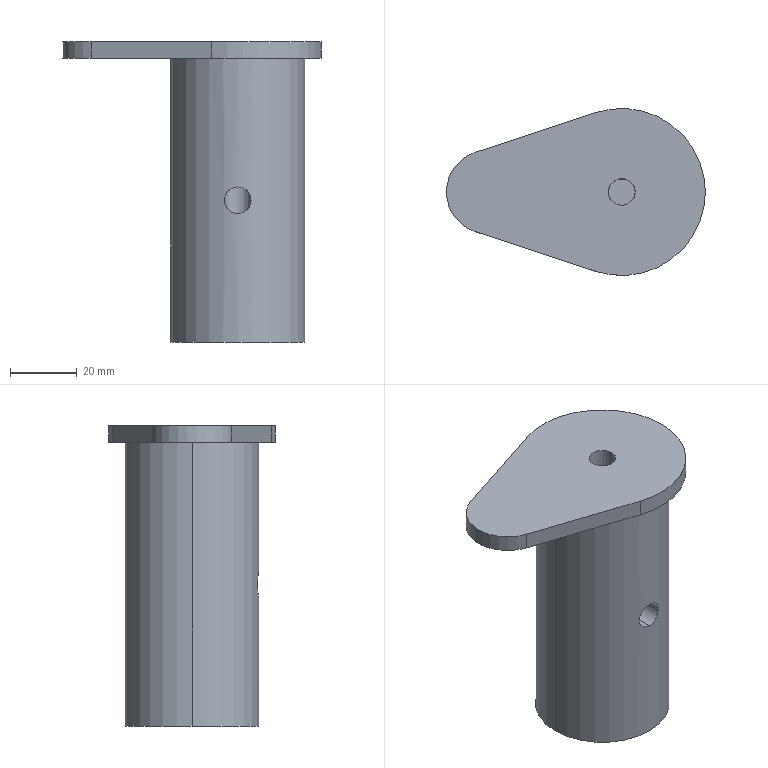Part | SolidWorks | features ICE 3, Extrusion 1 | 1 solid | 16 faces | box 77.5 x 50 x 90 mm | volume 116974 mm3 | cylinder 10 | plane 6 | commonest cylinder face diameters 8 x5 40 x2 50 x2 25 x1
STEP:
#1=CARTESIAN_POINT('',(0.,-20.,38.5));
#2=VERTEX_POINT('',#1);
#3=CARTESIAN_POINT('',(0.,-20.,46.5));
#4=VERTEX_POINT('',#3);
#5=CARTESIAN_POINT('',(0.,-20.,38.5));
#6=CARTESIAN_POINT('',(-0.2614,-20.,38.5));
#7=CARTESIAN_POINT('',(-0.5216,-19.995,38.525));
#8=CARTESIAN_POINT('',(-1.04,-19.975,38.628));
#9=CARTESIAN_POINT('',(-1.291,-19.96,38.705));
#10=CARTESIAN_POINT('',(-1.773,-19.923,38.905));
#11=CARTESIAN_POINT('',(-2.006,-19.9,39.03));
#12=CARTESIAN_POINT('',(-2.441,-19.852,39.321));
#13=CARTESIAN_POINT('',(-2.642,-19.826,39.486));
#14=CARTESIAN_POINT('',(-3.011,-19.773,39.854));
#15=CARTESIAN_POINT('',(-3.18,-19.746,40.059));
#16=CARTESIAN_POINT('',(-3.469,-19.697,40.492));
#17=CARTESIAN_POINT('',(-3.593,-19.675,40.722));
#18=CARTESIAN_POINT('',(-3.794,-19.637,41.207));
#19=CARTESIAN_POINT('',(-3.871,-19.622,41.46));
#20=CARTESIAN_POINT('',(-3.974,-19.601,41.972));
#21=CARTESIAN_POINT('',(-4.,-19.596,42.234));
#22=CARTESIAN_POINT('',(-4.,-19.596,42.762));
#23=CARTESIAN_POINT('',(-3.974,-19.601,43.022));
#24=CARTESIAN_POINT('',(-3.873,-19.622,43.535));
#25=CARTESIAN_POINT('',(-3.795,-19.637,43.79));
#26=CARTESIAN_POINT('',(-3.595,-19.674,44.273));
#27=CARTESIAN_POINT('',(-3.472,-19.697,44.503));
#28=CARTESIAN_POINT('',(-3.182,-19.746,44.938));
#29=CARTESIAN_POINT('',(-3.014,-19.772,45.143));
#30=CARTESIAN_POINT('',(-2.647,-19.825,45.511));
#31=CARTESIAN_POINT('',(-2.445,-19.851,45.676));
#32=CARTESIAN_POINT('',(-2.007,-19.9,45.97));
#33=CARTESIAN_POINT('',(-1.777,-19.922,46.093));
#34=CARTESIAN_POINT('',(-1.296,-19.959,46.293));
#35=CARTESIAN_POINT('',(-1.043,-19.974,46.371));
#36=CARTESIAN_POINT('',(-0.5264,-19.995,46.474));
#37=CARTESIAN_POINT('',(-0.2649,-20.,46.5));
#38=CARTESIAN_POINT('',(0.,-20.,46.5));
#39=B_SPLINE_CURVE_WITH_KNOTS('',3,(#5,#6,#7,#8,#9,#10,#11,#12,#13,#14,#15,#16,#17,#18,#19,#20,#21,#22,#23,#24,#25,#26,#27,#28,#29,#30,#31,#32,#33,#34,#35,#36,#37,#38),.UNSPECIFIED.,.F.,.F.,(4,2,2,2,2,2,2,2,2,2,2,2,2,2,2,2,4),(0.01254,0.01332,0.0141,0.01489,0.01567,0.01645,0.01724,0.01802,0.0188,0.01959,0.02037,0.02115,0.02194,0.02272,0.0235,0.02429,0.02507),.UNSPECIFIED.);
#40=EDGE_CURVE('',#2,#4,#39,.T.);
#41=ORIENTED_EDGE('',*,*,#40,.F.);
#42=CARTESIAN_POINT('',(0.,-4.,38.5));
#43=VERTEX_POINT('',#42);
#44=CARTESIAN_POINT('',(0.,-20.,38.5));
#45=DIRECTION('',(0.,1.,0.));
#46=VECTOR('',#45,1000.);
#47=LINE('',#44,#46);
#48=EDGE_CURVE('',#2,#43,#47,.T.);
#49=ORIENTED_EDGE('',*,*,#48,.T.);
#50=CARTESIAN_POINT('',(-4.,0.,42.5));
#51=VERTEX_POINT('',#50);
#52=CARTESIAN_POINT('',(-4.,0.,42.5));
#53=CARTESIAN_POINT('',(-4.,-2.343,40.157));
#54=CARTESIAN_POINT('',(-2.343,-4.,38.5));
#55=CARTESIAN_POINT('',(0.,-4.,38.5));
#56=(BOUNDED_CURVE()B_SPLINE_CURVE(3,(#52,#53,#54,#55),.UNSPECIFIED.,.F.,.T.)B_SPLINE_CURVE_WITH_KNOTS((4,4),(1.571,3.142),.UNSPECIFIED.)CURVE()GEOMETRIC_REPRESENTATION_ITEM()RATIONAL_B_SPLINE_CURVE((1.,0.8047,0.8047,1.))REPRESENTATION_ITEM(''));
#57=EDGE_CURVE('',#51,#43,#56,.T.);
#58=ORIENTED_EDGE('',*,*,#57,.F.);
#59=CARTESIAN_POINT('',(0.,-4.,46.5));
#60=VERTEX_POINT('',#59);
#61=CARTESIAN_POINT('',(0.,-4.,46.5));
#62=CARTESIAN_POINT('',(-2.343,-4.,46.5));
#63=CARTESIAN_POINT('',(-4.,-2.343,44.843));
#64=CARTESIAN_POINT('',(-4.,0.,42.5));
#65=(BOUNDED_CURVE()B_SPLINE_CURVE(3,(#61,#62,#63,#64),.UNSPECIFIED.,.F.,.F.)B_SPLINE_CURVE_WITH_KNOTS((4,4),(0.,1.571),.UNSPECIFIED.)CURVE()GEOMETRIC_REPRESENTATION_ITEM()RATIONAL_B_SPLINE_CURVE((1.,0.8047,0.8047,1.))REPRESENTATION_ITEM(''));
#66=EDGE_CURVE('',#60,#51,#65,.T.);
#67=ORIENTED_EDGE('',*,*,#66,.F.);
#68=CARTESIAN_POINT('',(0.,-20.,46.5));
#69=DIRECTION('',(0.,1.,0.));
#70=VECTOR('',#69,1000.);
#71=LINE('',#68,#70);
#72=EDGE_CURVE('',#4,#60,#71,.T.);
#73=ORIENTED_EDGE('',*,*,#72,.F.);
#74=EDGE_LOOP('',(#41,#49,#58,#67,#73));
#75=FACE_OUTER_BOUND('',#74,.T.);
#76=CARTESIAN_POINT('',(0.,-20.,42.5));
#77=DIRECTION('',(0.,1.,0.));
#78=DIRECTION('',(0.,0.,1.));
#79=AXIS2_PLACEMENT_3D('',#76,#77,#78);
#80=CYLINDRICAL_SURFACE('',#79,4.);
#81=ADVANCED_FACE('',(#75),#80,.F.);
#82=CARTESIAN_POINT('',(-4.,0.,30.));
#83=VERTEX_POINT('',#82);
#84=CARTESIAN_POINT('',(4.,0.,30.));
#85=VERTEX_POINT('',#84);
#86=CARTESIAN_POINT('',(0.,0.,30.));
#87=DIRECTION('',(0.,0.,1.));
#88=DIRECTION('',(1.,0.,0.));
#89=AXIS2_PLACEMENT_3D('',#86,#87,#88);
#90=CIRCLE('',#89,4.);
#91=EDGE_CURVE('',#83,#85,#90,.T.);
#92=ORIENTED_EDGE('',*,*,#91,.F.);
#93=CARTESIAN_POINT('',(-4.,0.,30.));
#94=DIRECTION('',(0.,0.,1.));
#95=VECTOR('',#94,1000.);
#96=LINE('',#93,#95);
#97=EDGE_CURVE('',#83,#51,#96,.T.);
#98=ORIENTED_EDGE('',*,*,#97,.T.);
#99=ORIENTED_EDGE('',*,*,#57,.T.);
#100=CARTESIAN_POINT('',(4.,0.,42.5));
#101=VERTEX_POINT('',#100);
#102=CARTESIAN_POINT('',(0.,-4.,38.5));
#103=CARTESIAN_POINT('',(2.343,-4.,38.5));
#104=CARTESIAN_POINT('',(4.,-2.343,40.157));
#105=CARTESIAN_POINT('',(4.,0.,42.5));
#106=(BOUNDED_CURVE()B_SPLINE_CURVE(3,(#102,#103,#104,#105),.UNSPECIFIED.,.F.,.T.)B_SPLINE_CURVE_WITH_KNOTS((4,4),(3.142,4.712),.UNSPECIFIED.)CURVE()GEOMETRIC_REPRESENTATION_ITEM()RATIONAL_B_SPLINE_CURVE((1.,0.8047,0.8047,1.))REPRESENTATION_ITEM(''));
#107=EDGE_CURVE('',#43,#101,#106,.T.);
#108=ORIENTED_EDGE('',*,*,#107,.T.);
#109=CARTESIAN_POINT('',(4.,0.,30.));
#110=DIRECTION('',(0.,0.,1.));
#111=VECTOR('',#110,1000.);
#112=LINE('',#109,#111);
#113=EDGE_CURVE('',#85,#101,#112,.T.);
#114=ORIENTED_EDGE('',*,*,#113,.F.);
#115=EDGE_LOOP('',(#92,#98,#99,#108,#114));
#116=FACE_OUTER_BOUND('',#115,.T.);
#117=CARTESIAN_POINT('',(0.,0.,30.));
#118=DIRECTION('',(0.,0.,1.));
#119=DIRECTION('',(1.,0.,0.));
#120=AXIS2_PLACEMENT_3D('',#117,#118,#119);
#121=CYLINDRICAL_SURFACE('',#120,4.);
#122=ADVANCED_FACE('',(#116),#121,.F.);
#123=CARTESIAN_POINT('',(4.,0.,42.5));
#124=CARTESIAN_POINT('',(4.,-2.343,44.843));
#125=CARTESIAN_POINT('',(2.343,-4.,46.5));
#126=CARTESIAN_POINT('',(0.,-4.,46.5));
#127=(BOUNDED_CURVE()B_SPLINE_CURVE(3,(#123,#124,#125,#126),.UNSPECIFIED.,.F.,.T.)B_SPLINE_CURVE_WITH_KNOTS((4,4),(4.712,6.283),.UNSPECIFIED.)CURVE()GEOMETRIC_REPRESENTATION_ITEM()RATIONAL_B_SPLINE_CURVE((1.,0.8047,0.8047,1.))REPRESENTATION_ITEM(''));
#128=EDGE_CURVE('',#101,#60,#127,.T.);
#129=ORIENTED_EDGE('',*,*,#128,.T.);
#130=ORIENTED_EDGE('',*,*,#66,.T.);
#131=CARTESIAN_POINT('',(-4.,0.,90.));
#132=VERTEX_POINT('',#131);
#133=CARTESIAN_POINT('',(-4.,0.,30.));
#134=DIRECTION('',(0.,0.,1.));
#135=VECTOR('',#134,1000.);
#136=LINE('',#133,#135);
#137=EDGE_CURVE('',#51,#132,#136,.T.);
#138=ORIENTED_EDGE('',*,*,#137,.T.);
#139=CARTESIAN_POINT('',(4.,0.,90.));
#140=VERTEX_POINT('',#139);
#141=CARTESIAN_POINT('',(0.,0.,90.));
#142=DIRECTION('',(0.,0.,1.));
#143=DIRECTION('',(1.,0.,0.));
#144=AXIS2_PLACEMENT_3D('',#141,#142,#143);
#145=CIRCLE('',#144,4.);
#146=EDGE_CURVE('',#132,#140,#145,.T.);
#147=ORIENTED_EDGE('',*,*,#146,.T.);
#148=CARTESIAN_POINT('',(4.,0.,30.));
#149=DIRECTION('',(0.,0.,1.));
#150=VECTOR('',#149,1000.);
#151=LINE('',#148,#150);
#152=EDGE_CURVE('',#101,#140,#151,.T.);
#153=ORIENTED_EDGE('',*,*,#152,.F.);
#154=EDGE_LOOP('',(#129,#130,#138,#147,#153));
#155=FACE_OUTER_BOUND('',#154,.T.);
#156=CARTESIAN_POINT('',(0.,0.,30.));
#157=DIRECTION('',(0.,0.,1.));
#158=DIRECTION('',(1.,0.,0.));
#159=AXIS2_PLACEMENT_3D('',#156,#157,#158);
#160=CYLINDRICAL_SURFACE('',#159,4.);
#161=ADVANCED_FACE('',(#155),#160,.F.);
#162=CARTESIAN_POINT('',(-7.813,-23.748,85.));
#163=VERTEX_POINT('',#162);
#164=CARTESIAN_POINT('',(25.,0.,85.));
#165=VERTEX_POINT('',#164);
#166=CARTESIAN_POINT('',(0.,0.,85.));
#167=DIRECTION('',(0.,0.,1.));
#168=DIRECTION('',(1.,0.,0.));
#169=AXIS2_PLACEMENT_3D('',#166,#167,#168);
#170=CIRCLE('',#169,25.);
#171=EDGE_CURVE('',#163,#165,#170,.T.);
#172=ORIENTED_EDGE('',*,*,#171,.T.);
#173=CARTESIAN_POINT('',(25.,0.,90.));
#174=VERTEX_POINT('',#173);
#175=CARTESIAN_POINT('',(25.,0.,85.));
#176=DIRECTION('',(0.,0.,1.));
#177=VECTOR('',#176,1000.);
#178=LINE('',#175,#177);
#179=EDGE_CURVE('',#165,#174,#178,.T.);
#180=ORIENTED_EDGE('',*,*,#179,.T.);
#181=CARTESIAN_POINT('',(-7.813,-23.748,90.));
#182=VERTEX_POINT('',#181);
#183=CARTESIAN_POINT('',(0.,0.,90.));
#184=DIRECTION('',(0.,0.,1.));
#185=DIRECTION('',(1.,0.,0.));
#186=AXIS2_PLACEMENT_3D('',#183,#184,#185);
#187=CIRCLE('',#186,25.);
#188=EDGE_CURVE('',#182,#174,#187,.T.);
#189=ORIENTED_EDGE('',*,*,#188,.F.);
#190=CARTESIAN_POINT('',(-7.813,-23.748,85.));
#191=DIRECTION('',(0.,0.,1.));
#192=VECTOR('',#191,1000.);
#193=LINE('',#190,#192);
#194=EDGE_CURVE('',#163,#182,#193,.T.);
#195=ORIENTED_EDGE('',*,*,#194,.F.);
#196=EDGE_LOOP('',(#172,#180,#189,#195));
#197=FACE_OUTER_BOUND('',#196,.T.);
#198=CARTESIAN_POINT('',(0.,0.,85.));
#199=DIRECTION('',(0.,0.,1.));
#200=DIRECTION('',(1.,0.,0.));
#201=AXIS2_PLACEMENT_3D('',#198,#199,#200);
#202=CYLINDRICAL_SURFACE('',#201,25.);
#203=ADVANCED_FACE('',(#197),#202,.T.);
#204=CARTESIAN_POINT('',(20.,0.,85.));
#205=VERTEX_POINT('',#204);
#206=CARTESIAN_POINT('',(-20.,0.,85.));
#207=VERTEX_POINT('',#206);
#208=CARTESIAN_POINT('',(0.,0.,85.));
#209=DIRECTION('',(0.,0.,1.));
#210=DIRECTION('',(1.,0.,0.));
#211=AXIS2_PLACEMENT_3D('',#208,#209,#210);
#212=CIRCLE('',#211,20.);
#213=EDGE_CURVE('',#205,#207,#212,.T.);
#214=ORIENTED_EDGE('',*,*,#213,.F.);
#215=CARTESIAN_POINT('',(20.,0.,0.));
#216=VERTEX_POINT('',#215);
#217=CARTESIAN_POINT('',(20.,0.,90.));
#218=DIRECTION('',(0.,0.,-1.));
#219=VECTOR('',#218,1000.);
#220=LINE('',#217,#219);
#221=EDGE_CURVE('',#205,#216,#220,.T.);
#222=ORIENTED_EDGE('',*,*,#221,.T.);
#223=CARTESIAN_POINT('',(-20.,0.,0.));
#224=VERTEX_POINT('',#223);
#225=CARTESIAN_POINT('',(0.,0.,0.));
#226=DIRECTION('',(0.,0.,1.));
#227=DIRECTION('',(1.,0.,0.));
#228=AXIS2_PLACEMENT_3D('',#225,#226,#227);
#229=CIRCLE('',#228,20.);
#230=EDGE_CURVE('',#216,#224,#229,.T.);
#231=ORIENTED_EDGE('',*,*,#230,.T.);
#232=CARTESIAN_POINT('',(-20.,0.,90.));
#233=DIRECTION('',(0.,0.,-1.));
#234=VECTOR('',#233,1000.);
#235=LINE('',#232,#234);
#236=EDGE_CURVE('',#207,#224,#235,.T.);
#237=ORIENTED_EDGE('',*,*,#236,.F.);
#238=EDGE_LOOP('',(#214,#222,#231,#237));
#239=FACE_OUTER_BOUND('',#238,.T.);
#240=CARTESIAN_POINT('',(0.,0.,90.));
#241=DIRECTION('',(0.,0.,-1.));
#242=DIRECTION('',(-1.,0.,0.));
#243=AXIS2_PLACEMENT_3D('',#240,#241,#242);
#244=CYLINDRICAL_SURFACE('',#243,20.);
#245=ADVANCED_FACE('',(#239),#244,.T.);
#246=ORIENTED_EDGE('',*,*,#221,.F.);
#247=CARTESIAN_POINT('',(0.,0.,85.));
#248=DIRECTION('',(0.,0.,1.));
#249=DIRECTION('',(1.,0.,0.));
#250=AXIS2_PLACEMENT_3D('',#247,#248,#249);
#251=CIRCLE('',#250,20.);
#252=EDGE_CURVE('',#207,#205,#251,.T.);
#253=ORIENTED_EDGE('',*,*,#252,.F.);
#254=ORIENTED_EDGE('',*,*,#236,.T.);
#255=CARTESIAN_POINT('',(0.,0.,0.));
#256=DIRECTION('',(0.,0.,1.));
#257=DIRECTION('',(1.,0.,0.));
#258=AXIS2_PLACEMENT_3D('',#255,#256,#257);
#259=CIRCLE('',#258,20.);
#260=EDGE_CURVE('',#224,#216,#259,.T.);
#261=ORIENTED_EDGE('',*,*,#260,.T.);
#262=EDGE_LOOP('',(#246,#253,#254,#261));
#263=FACE_OUTER_BOUND('',#262,.T.);
#264=CARTESIAN_POINT('',(0.,-20.,46.5));
#265=CARTESIAN_POINT('',(0.265,-20.,46.5));
#266=CARTESIAN_POINT('',(0.5255,-19.995,46.474));
#267=CARTESIAN_POINT('',(1.038,-19.975,46.372));
#268=CARTESIAN_POINT('',(1.292,-19.96,46.295));
#269=CARTESIAN_POINT('',(1.776,-19.922,46.094));
#270=CARTESIAN_POINT('',(2.006,-19.9,45.971));
#271=CARTESIAN_POINT('',(2.44,-19.852,45.68));
#272=CARTESIAN_POINT('',(2.645,-19.825,45.512));
#273=CARTESIAN_POINT('',(3.013,-19.773,45.144));
#274=CARTESIAN_POINT('',(3.178,-19.746,44.943));
#275=CARTESIAN_POINT('',(3.471,-19.697,44.506));
#276=CARTESIAN_POINT('',(3.595,-19.675,44.274));
#277=CARTESIAN_POINT('',(3.794,-19.637,43.793));
#278=CARTESIAN_POINT('',(3.871,-19.622,43.54));
#279=CARTESIAN_POINT('',(3.974,-19.601,43.023));
#280=CARTESIAN_POINT('',(4.,-19.596,42.763));
#281=CARTESIAN_POINT('',(4.,-19.596,42.24));
#282=CARTESIAN_POINT('',(3.974,-19.601,41.974));
#283=CARTESIAN_POINT('',(3.871,-19.622,41.461));
#284=CARTESIAN_POINT('',(3.796,-19.637,41.211));
#285=CARTESIAN_POINT('',(3.595,-19.675,40.726));
#286=CARTESIAN_POINT('',(3.47,-19.697,40.493));
#287=CARTESIAN_POINT('',(3.18,-19.746,40.06));
#288=CARTESIAN_POINT('',(3.014,-19.772,39.857));
#289=CARTESIAN_POINT('',(2.642,-19.826,39.485));
#290=CARTESIAN_POINT('',(2.441,-19.852,39.32));
#291=CARTESIAN_POINT('',(2.008,-19.9,39.031));
#292=CARTESIAN_POINT('',(1.774,-19.923,38.905));
#293=CARTESIAN_POINT('',(1.29,-19.96,38.705));
#294=CARTESIAN_POINT('',(1.041,-19.975,38.629));
#295=CARTESIAN_POINT('',(0.5269,-19.995,38.526));
#296=CARTESIAN_POINT('',(0.2614,-20.,38.5));
#297=CARTESIAN_POINT('',(0.,-20.,38.5));
#298=B_SPLINE_CURVE_WITH_KNOTS('',3,(#264,#265,#266,#267,#268,#269,#270,#271,#272,#273,#274,#275,#276,#277,#278,#279,#280,#281,#282,#283,#284,#285,#286,#287,#288,#289,#290,#291,#292,#293,#294,#295,#296,#297),.UNSPECIFIED.,.F.,.F.,(4,2,2,2,2,2,2,2,2,2,2,2,2,2,2,2,4),(0.,0.0007836,0.001567,0.002351,0.003134,0.003918,0.004702,0.005485,0.006269,0.007052,0.007836,0.00862,0.009403,0.01019,0.01097,0.01175,0.01254),.UNSPECIFIED.);
#299=EDGE_CURVE('',#4,#2,#298,.T.);
#300=ORIENTED_EDGE('',*,*,#299,.T.);
#301=ORIENTED_EDGE('',*,*,#40,.T.);
#302=EDGE_LOOP('',(#300,#301));
#303=FACE_BOUND('',#302,.T.);
#304=CARTESIAN_POINT('',(0.,0.,90.));
#305=DIRECTION('',(0.,0.,-1.));
#306=DIRECTION('',(-1.,0.,0.));
#307=AXIS2_PLACEMENT_3D('',#304,#305,#306);
#308=CYLINDRICAL_SURFACE('',#307,20.);
#309=ADVANCED_FACE('',(#263,#303),#308,.T.);
#310=ORIENTED_EDGE('',*,*,#260,.F.);
#311=ORIENTED_EDGE('',*,*,#230,.F.);
#312=EDGE_LOOP('',(#310,#311));
#313=FACE_OUTER_BOUND('',#312,.T.);
#314=CARTESIAN_POINT('',(0.,0.,0.));
#315=DIRECTION('',(0.,0.,1.));
#316=DIRECTION('',(1.,0.,0.));
#317=AXIS2_PLACEMENT_3D('',#314,#315,#316);
#318=PLANE('',#317);
#319=ADVANCED_FACE('',(#313),#318,.F.);
#320=CARTESIAN_POINT('',(-43.906,11.874,85.));
#321=VERTEX_POINT('',#320);
#322=CARTESIAN_POINT('',(-43.906,-11.874,85.));
#323=VERTEX_POINT('',#322);
#324=CARTESIAN_POINT('',(-40.,0.,85.));
#325=DIRECTION('',(0.,0.,1.));
#326=DIRECTION('',(1.,0.,0.));
#327=AXIS2_PLACEMENT_3D('',#324,#325,#326);
#328=CIRCLE('',#327,12.5);
#329=EDGE_CURVE('',#321,#323,#328,.T.);
#330=ORIENTED_EDGE('',*,*,#329,.F.);
#331=CARTESIAN_POINT('',(-7.812,23.748,85.));
#332=VERTEX_POINT('',#331);
#333=CARTESIAN_POINT('',(-43.906,11.874,85.));
#334=DIRECTION('',(-0.9499,-0.3125,0.));
#335=VECTOR('',#334,1000.);
#336=LINE('',#333,#335);
#337=EDGE_CURVE('',#332,#321,#336,.T.);
#338=ORIENTED_EDGE('',*,*,#337,.F.);
#339=CARTESIAN_POINT('',(0.,0.,85.));
#340=DIRECTION('',(0.,0.,1.));
#341=DIRECTION('',(1.,0.,0.));
#342=AXIS2_PLACEMENT_3D('',#339,#340,#341);
#343=CIRCLE('',#342,25.);
#344=EDGE_CURVE('',#165,#332,#343,.T.);
#345=ORIENTED_EDGE('',*,*,#344,.F.);
#346=ORIENTED_EDGE('',*,*,#171,.F.);
#347=CARTESIAN_POINT('',(-7.812,-23.748,85.));
#348=DIRECTION('',(0.9499,-0.3125,0.));
#349=VECTOR('',#348,1000.);
#350=LINE('',#347,#349);
#351=EDGE_CURVE('',#323,#163,#350,.T.);
#352=ORIENTED_EDGE('',*,*,#351,.F.);
#353=EDGE_LOOP('',(#330,#338,#345,#346,#352));
#354=FACE_OUTER_BOUND('',#353,.T.);
#355=ORIENTED_EDGE('',*,*,#252,.T.);
#356=ORIENTED_EDGE('',*,*,#213,.T.);
#357=EDGE_LOOP('',(#355,#356));
#358=FACE_BOUND('',#357,.T.);
#359=CARTESIAN_POINT('',(-40.,0.,85.));
#360=DIRECTION('',(0.,0.,1.));
#361=DIRECTION('',(1.,0.,0.));
#362=AXIS2_PLACEMENT_3D('',#359,#360,#361);
#363=PLANE('',#362);
#364=ADVANCED_FACE('',(#354,#358),#363,.F.);
#365=CARTESIAN_POINT('',(-43.906,11.874,90.));
#366=VERTEX_POINT('',#365);
#367=CARTESIAN_POINT('',(-43.906,-11.874,90.));
#368=VERTEX_POINT('',#367);
#369=CARTESIAN_POINT('',(-40.,0.,90.));
#370=DIRECTION('',(0.,0.,1.));
#371=DIRECTION('',(1.,0.,0.));
#372=AXIS2_PLACEMENT_3D('',#369,#370,#371);
#373=CIRCLE('',#372,12.5);
#374=EDGE_CURVE('',#366,#368,#373,.T.);
#375=ORIENTED_EDGE('',*,*,#374,.F.);
#376=CARTESIAN_POINT('',(-43.906,11.874,85.));
#377=DIRECTION('',(0.,0.,1.));
#378=VECTOR('',#377,1000.);
#379=LINE('',#376,#378);
#380=EDGE_CURVE('',#321,#366,#379,.T.);
#381=ORIENTED_EDGE('',*,*,#380,.F.);
#382=ORIENTED_EDGE('',*,*,#329,.T.);
#383=CARTESIAN_POINT('',(-43.906,-11.874,85.));
#384=DIRECTION('',(0.,0.,1.));
#385=VECTOR('',#384,1000.);
#386=LINE('',#383,#385);
#387=EDGE_CURVE('',#323,#368,#386,.T.);
#388=ORIENTED_EDGE('',*,*,#387,.T.);
#389=EDGE_LOOP('',(#375,#381,#382,#388));
#390=FACE_OUTER_BOUND('',#389,.T.);
#391=CARTESIAN_POINT('',(-40.,0.,85.));
#392=DIRECTION('',(0.,0.,1.));
#393=DIRECTION('',(1.,0.,0.));
#394=AXIS2_PLACEMENT_3D('',#391,#392,#393);
#395=CYLINDRICAL_SURFACE('',#394,12.5);
#396=ADVANCED_FACE('',(#390),#395,.T.);
#397=CARTESIAN_POINT('',(-7.812,23.748,90.));
#398=VERTEX_POINT('',#397);
#399=CARTESIAN_POINT('',(-43.906,11.874,90.));
#400=DIRECTION('',(-0.9499,-0.3125,0.));
#401=VECTOR('',#400,1000.);
#402=LINE('',#399,#401);
#403=EDGE_CURVE('',#398,#366,#402,.T.);
#404=ORIENTED_EDGE('',*,*,#403,.F.);
#405=CARTESIAN_POINT('',(-7.812,23.748,85.));
#406=DIRECTION('',(0.,0.,1.));
#407=VECTOR('',#406,1000.);
#408=LINE('',#405,#407);
#409=EDGE_CURVE('',#332,#398,#408,.T.);
#410=ORIENTED_EDGE('',*,*,#409,.F.);
#411=ORIENTED_EDGE('',*,*,#337,.T.);
#412=ORIENTED_EDGE('',*,*,#380,.T.);
#413=EDGE_LOOP('',(#404,#410,#411,#412));
#414=FACE_OUTER_BOUND('',#413,.T.);
#415=CARTESIAN_POINT('',(-43.906,11.874,85.));
#416=DIRECTION('',(-0.3125,0.9499,0.));
#417=DIRECTION('',(-0.9499,-0.3125,0.));
#418=AXIS2_PLACEMENT_3D('',#415,#416,#417);
#419=PLANE('',#418);
#420=ADVANCED_FACE('',(#414),#419,.T.);
#421=ORIENTED_EDGE('',*,*,#179,.F.);
#422=ORIENTED_EDGE('',*,*,#344,.T.);
#423=ORIENTED_EDGE('',*,*,#409,.T.);
#424=CARTESIAN_POINT('',(0.,0.,90.));
#425=DIRECTION('',(0.,0.,1.));
#426=DIRECTION('',(1.,0.,0.));
#427=AXIS2_PLACEMENT_3D('',#424,#425,#426);
#428=CIRCLE('',#427,25.);
#429=EDGE_CURVE('',#174,#398,#428,.T.);
#430=ORIENTED_EDGE('',*,*,#429,.F.);
#431=EDGE_LOOP('',(#421,#422,#423,#430));
#432=FACE_OUTER_BOUND('',#431,.T.);
#433=CARTESIAN_POINT('',(0.,0.,85.));
#434=DIRECTION('',(0.,0.,1.));
#435=DIRECTION('',(1.,0.,0.));
#436=AXIS2_PLACEMENT_3D('',#433,#434,#435);
#437=CYLINDRICAL_SURFACE('',#436,25.);
#438=ADVANCED_FACE('',(#432),#437,.T.);
#439=CARTESIAN_POINT('',(-7.812,-23.748,90.));
#440=DIRECTION('',(0.9499,-0.3125,0.));
#441=VECTOR('',#440,1000.);
#442=LINE('',#439,#441);
#443=EDGE_CURVE('',#368,#182,#442,.T.);
#444=ORIENTED_EDGE('',*,*,#443,.F.);
#445=ORIENTED_EDGE('',*,*,#387,.F.);
#446=ORIENTED_EDGE('',*,*,#351,.T.);
#447=ORIENTED_EDGE('',*,*,#194,.T.);
#448=EDGE_LOOP('',(#444,#445,#446,#447));
#449=FACE_OUTER_BOUND('',#448,.T.);
#450=CARTESIAN_POINT('',(-7.812,-23.748,85.));
#451=DIRECTION('',(-0.3125,-0.9499,0.));
#452=DIRECTION('',(0.9499,-0.3125,0.));
#453=AXIS2_PLACEMENT_3D('',#450,#451,#452);
#454=PLANE('',#453);
#455=ADVANCED_FACE('',(#449),#454,.T.);
#456=CARTESIAN_POINT('',(0.,0.,90.));
#457=DIRECTION('',(0.,0.,1.));
#458=DIRECTION('',(1.,0.,0.));
#459=AXIS2_PLACEMENT_3D('',#456,#457,#458);
#460=CIRCLE('',#459,4.);
#461=EDGE_CURVE('',#140,#132,#460,.T.);
#462=ORIENTED_EDGE('',*,*,#461,.F.);
#463=ORIENTED_EDGE('',*,*,#146,.F.);
#464=EDGE_LOOP('',(#462,#463));
#465=FACE_BOUND('',#464,.T.);
#466=ORIENTED_EDGE('',*,*,#374,.T.);
#467=ORIENTED_EDGE('',*,*,#443,.T.);
#468=ORIENTED_EDGE('',*,*,#188,.T.);
#469=ORIENTED_EDGE('',*,*,#429,.T.);
#470=ORIENTED_EDGE('',*,*,#403,.T.);
#471=EDGE_LOOP('',(#466,#467,#468,#469,#470));
#472=FACE_OUTER_BOUND('',#471,.T.);
#473=CARTESIAN_POINT('',(0.,0.,90.));
#474=DIRECTION('',(0.,0.,1.));
#475=DIRECTION('',(1.,0.,0.));
#476=AXIS2_PLACEMENT_3D('',#473,#474,#475);
#477=PLANE('',#476);
#478=ADVANCED_FACE('',(#465,#472),#477,.T.);
#479=ORIENTED_EDGE('',*,*,#97,.F.);
#480=CARTESIAN_POINT('',(0.,0.,30.));
#481=DIRECTION('',(0.,0.,1.));
#482=DIRECTION('',(1.,0.,0.));
#483=AXIS2_PLACEMENT_3D('',#480,#481,#482);
#484=CIRCLE('',#483,4.);
#485=EDGE_CURVE('',#85,#83,#484,.T.);
#486=ORIENTED_EDGE('',*,*,#485,.F.);
#487=ORIENTED_EDGE('',*,*,#113,.T.);
#488=ORIENTED_EDGE('',*,*,#152,.T.);
#489=ORIENTED_EDGE('',*,*,#461,.T.);
#490=ORIENTED_EDGE('',*,*,#137,.F.);
#491=EDGE_LOOP('',(#479,#486,#487,#488,#489,#490));
#492=FACE_OUTER_BOUND('',#491,.T.);
#493=CARTESIAN_POINT('',(0.,0.,30.));
#494=DIRECTION('',(0.,0.,1.));
#495=DIRECTION('',(1.,0.,0.));
#496=AXIS2_PLACEMENT_3D('',#493,#494,#495);
#497=CYLINDRICAL_SURFACE('',#496,4.);
#498=ADVANCED_FACE('',(#492),#497,.F.);
#499=ORIENTED_EDGE('',*,*,#485,.T.);
#500=ORIENTED_EDGE('',*,*,#91,.T.);
#501=EDGE_LOOP('',(#499,#500));
#502=FACE_OUTER_BOUND('',#501,.T.);
#503=CARTESIAN_POINT('',(0.,0.,30.));
#504=DIRECTION('',(0.,0.,1.));
#505=DIRECTION('',(1.,0.,0.));
#506=AXIS2_PLACEMENT_3D('',#503,#504,#505);
#507=PLANE('',#506);
#508=ADVANCED_FACE('',(#502),#507,.T.);
#509=ORIENTED_EDGE('',*,*,#48,.F.);
#510=ORIENTED_EDGE('',*,*,#299,.F.);
#511=ORIENTED_EDGE('',*,*,#72,.T.);
#512=ORIENTED_EDGE('',*,*,#128,.F.);
#513=ORIENTED_EDGE('',*,*,#107,.F.);
#514=EDGE_LOOP('',(#509,#510,#511,#512,#513));
#515=FACE_OUTER_BOUND('',#514,.T.);
#516=CARTESIAN_POINT('',(0.,-20.,42.5));
#517=DIRECTION('',(0.,1.,0.));
#518=DIRECTION('',(0.,0.,1.));
#519=AXIS2_PLACEMENT_3D('',#516,#517,#518);
#520=CYLINDRICAL_SURFACE('',#519,4.);
#521=ADVANCED_FACE('',(#515),#520,.F.);
#522=CLOSED_SHELL('',(#81,#122,#161,#203,#245,#309,#319,#364,#396,#420,#438,#455,#478,#498,#508,#521));
#523=MANIFOLD_SOLID_BREP('',#522);
#524=CARTESIAN_POINT('',(0.,0.,0.));
#525=DIRECTION('',(0.,0.,1.));
#526=DIRECTION('',(1.,0.,0.));
#527=AXIS2_PLACEMENT_3D('',#524,#525,#526);
#528=(LENGTH_UNIT()NAMED_UNIT(*)SI_UNIT(.MILLI.,.METRE.));
#529=UNCERTAINTY_MEASURE_WITH_UNIT(LENGTH_MEASURE(0.00001),#528,'','');
#530=(NAMED_UNIT(*)PLANE_ANGLE_UNIT()SI_UNIT($,.RADIAN.));
#531=(NAMED_UNIT(*)SI_UNIT($,.STERADIAN.)SOLID_ANGLE_UNIT());
#532=(GEOMETRIC_REPRESENTATION_CONTEXT(3)GLOBAL_UNCERTAINTY_ASSIGNED_CONTEXT((#529))GLOBAL_UNIT_ASSIGNED_CONTEXT((#528,#530,#531))REPRESENTATION_CONTEXT('',''));
#533=ADVANCED_BREP_SHAPE_REPRESENTATION('',(#523,#527),#532);